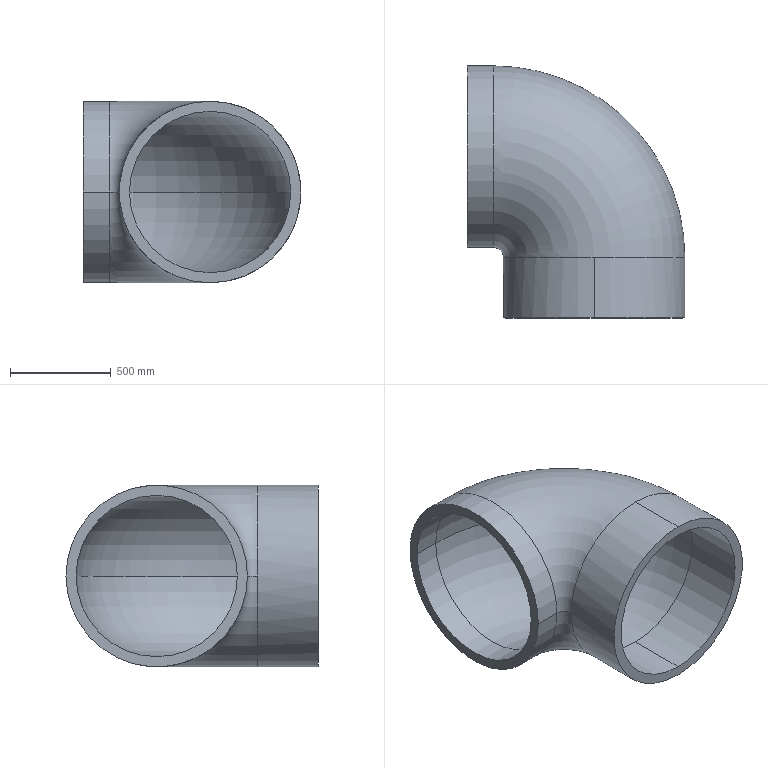Part | SolidWorks | features ICE 3, MoveFace 3, Extrusion 1, Sweep 1 | 1 solid | 14 faces | box 1080 x 1250 x 900 mm | volume 162277153 mm3 | cylinder 8 | torus 4 | plane 2 | commonest cylinder face diameters 800 x4 900 x4
STEP:
#1=CARTESIAN_POINT('',(0.,500.,-400.));
#2=VERTEX_POINT('',#1);
#3=CARTESIAN_POINT('',(400.,500.,0.));
#4=VERTEX_POINT('',#3);
#5=CARTESIAN_POINT('',(0.,500.,0.));
#6=DIRECTION('',(0.,-1.,0.));
#7=DIRECTION('',(0.,0.,1.));
#8=AXIS2_PLACEMENT_3D('',#5,#6,#7);
#9=CIRCLE('',#8,400.);
#10=EDGE_CURVE('',#2,#4,#9,.T.);
#11=ORIENTED_EDGE('',*,*,#10,.T.);
#12=CARTESIAN_POINT('',(-500.,1400.,0.));
#13=VERTEX_POINT('',#12);
#14=CARTESIAN_POINT('',(-500.,500.,0.));
#15=DIRECTION('',(0.,0.,1.));
#16=DIRECTION('',(1.,0.,0.));
#17=AXIS2_PLACEMENT_3D('',#14,#15,#16);
#18=CIRCLE('',#17,900.);
#19=EDGE_CURVE('',#4,#13,#18,.T.);
#20=ORIENTED_EDGE('',*,*,#19,.T.);
#21=CARTESIAN_POINT('',(-500.,600.,0.));
#22=VERTEX_POINT('',#21);
#23=CARTESIAN_POINT('',(-500.,1000.,0.));
#24=DIRECTION('',(1.,0.,0.));
#25=DIRECTION('',(0.,0.,1.));
#26=AXIS2_PLACEMENT_3D('',#23,#24,#25);
#27=CIRCLE('',#26,400.);
#28=EDGE_CURVE('',#22,#13,#27,.T.);
#29=ORIENTED_EDGE('',*,*,#28,.F.);
#30=CARTESIAN_POINT('',(-400.,500.,0.));
#31=VERTEX_POINT('',#30);
#32=CARTESIAN_POINT('',(-500.,500.,0.));
#33=DIRECTION('',(0.,0.,1.));
#34=DIRECTION('',(1.,0.,0.));
#35=AXIS2_PLACEMENT_3D('',#32,#33,#34);
#36=CIRCLE('',#35,100.);
#37=EDGE_CURVE('',#31,#22,#36,.T.);
#38=ORIENTED_EDGE('',*,*,#37,.F.);
#39=CARTESIAN_POINT('',(0.,500.,0.));
#40=DIRECTION('',(0.,-1.,0.));
#41=DIRECTION('',(0.,0.,1.));
#42=AXIS2_PLACEMENT_3D('',#39,#40,#41);
#43=CIRCLE('',#42,400.);
#44=EDGE_CURVE('',#31,#2,#43,.T.);
#45=ORIENTED_EDGE('',*,*,#44,.T.);
#46=EDGE_LOOP('',(#11,#20,#29,#38,#45));
#47=FACE_OUTER_BOUND('',#46,.T.);
#48=CARTESIAN_POINT('',(-500.,500.,0.));
#49=DIRECTION('',(0.,0.,1.));
#50=DIRECTION('',(1.,0.,0.));
#51=AXIS2_PLACEMENT_3D('',#48,#49,#50);
#52=TOROIDAL_SURFACE('',#51,500.,400.);
#53=ADVANCED_FACE('',(#47),#52,.F.);
#54=CARTESIAN_POINT('',(0.,500.,450.));
#55=VERTEX_POINT('',#54);
#56=CARTESIAN_POINT('',(450.,500.,0.));
#57=VERTEX_POINT('',#56);
#58=CARTESIAN_POINT('',(0.,500.,0.));
#59=DIRECTION('',(0.,1.,0.));
#60=DIRECTION('',(0.,0.,1.));
#61=AXIS2_PLACEMENT_3D('',#58,#59,#60);
#62=CIRCLE('',#61,450.);
#63=EDGE_CURVE('',#55,#57,#62,.T.);
#64=ORIENTED_EDGE('',*,*,#63,.T.);
#65=CARTESIAN_POINT('',(-500.,1450.,0.));
#66=VERTEX_POINT('',#65);
#67=CARTESIAN_POINT('',(-500.,500.,0.));
#68=DIRECTION('',(0.,0.,1.));
#69=DIRECTION('',(1.,0.,0.));
#70=AXIS2_PLACEMENT_3D('',#67,#68,#69);
#71=CIRCLE('',#70,950.);
#72=EDGE_CURVE('',#57,#66,#71,.T.);
#73=ORIENTED_EDGE('',*,*,#72,.T.);
#74=CARTESIAN_POINT('',(-500.,550.,0.));
#75=VERTEX_POINT('',#74);
#76=CARTESIAN_POINT('',(-500.,1000.,0.));
#77=DIRECTION('',(-1.,0.,0.));
#78=DIRECTION('',(0.,0.,1.));
#79=AXIS2_PLACEMENT_3D('',#76,#77,#78);
#80=CIRCLE('',#79,450.);
#81=EDGE_CURVE('',#75,#66,#80,.T.);
#82=ORIENTED_EDGE('',*,*,#81,.F.);
#83=CARTESIAN_POINT('',(-450.,500.,0.));
#84=VERTEX_POINT('',#83);
#85=CARTESIAN_POINT('',(-500.,500.,0.));
#86=DIRECTION('',(0.,0.,1.));
#87=DIRECTION('',(1.,0.,0.));
#88=AXIS2_PLACEMENT_3D('',#85,#86,#87);
#89=CIRCLE('',#88,50.);
#90=EDGE_CURVE('',#84,#75,#89,.T.);
#91=ORIENTED_EDGE('',*,*,#90,.F.);
#92=CARTESIAN_POINT('',(0.,500.,0.));
#93=DIRECTION('',(0.,1.,0.));
#94=DIRECTION('',(0.,0.,1.));
#95=AXIS2_PLACEMENT_3D('',#92,#93,#94);
#96=CIRCLE('',#95,450.);
#97=EDGE_CURVE('',#84,#55,#96,.T.);
#98=ORIENTED_EDGE('',*,*,#97,.T.);
#99=EDGE_LOOP('',(#64,#73,#82,#91,#98));
#100=FACE_OUTER_BOUND('',#99,.T.);
#101=CARTESIAN_POINT('',(-500.,500.,0.));
#102=DIRECTION('',(0.,0.,1.));
#103=DIRECTION('',(1.,0.,0.));
#104=AXIS2_PLACEMENT_3D('',#101,#102,#103);
#105=TOROIDAL_SURFACE('',#104,500.,450.);
#106=ADVANCED_FACE('',(#100),#105,.T.);
#107=CARTESIAN_POINT('',(0.,500.,400.));
#108=VERTEX_POINT('',#107);
#109=CARTESIAN_POINT('',(0.,500.,0.));
#110=DIRECTION('',(0.,-1.,0.));
#111=DIRECTION('',(0.,0.,1.));
#112=AXIS2_PLACEMENT_3D('',#109,#110,#111);
#113=CIRCLE('',#112,400.);
#114=EDGE_CURVE('',#108,#31,#113,.T.);
#115=ORIENTED_EDGE('',*,*,#114,.F.);
#116=CARTESIAN_POINT('',(0.,200.,400.));
#117=VERTEX_POINT('',#116);
#118=CARTESIAN_POINT('',(0.,750.,400.));
#119=DIRECTION('',(0.,-1.,0.));
#120=VECTOR('',#119,1000.);
#121=LINE('',#118,#120);
#122=EDGE_CURVE('',#108,#117,#121,.T.);
#123=ORIENTED_EDGE('',*,*,#122,.T.);
#124=CARTESIAN_POINT('',(0.,200.,-400.));
#125=VERTEX_POINT('',#124);
#126=CARTESIAN_POINT('',(0.,200.,0.));
#127=DIRECTION('',(0.,1.,0.));
#128=DIRECTION('',(0.,0.,1.));
#129=AXIS2_PLACEMENT_3D('',#126,#127,#128);
#130=CIRCLE('',#129,400.);
#131=EDGE_CURVE('',#125,#117,#130,.T.);
#132=ORIENTED_EDGE('',*,*,#131,.F.);
#133=CARTESIAN_POINT('',(0.,750.,-400.));
#134=DIRECTION('',(0.,-1.,0.));
#135=VECTOR('',#134,1000.);
#136=LINE('',#133,#135);
#137=EDGE_CURVE('',#2,#125,#136,.T.);
#138=ORIENTED_EDGE('',*,*,#137,.F.);
#139=ORIENTED_EDGE('',*,*,#44,.F.);
#140=EDGE_LOOP('',(#115,#123,#132,#138,#139));
#141=FACE_OUTER_BOUND('',#140,.T.);
#142=CARTESIAN_POINT('',(0.,750.,0.));
#143=DIRECTION('',(0.,-1.,0.));
#144=DIRECTION('',(0.,0.,-1.));
#145=AXIS2_PLACEMENT_3D('',#142,#143,#144);
#146=CYLINDRICAL_SURFACE('',#145,400.);
#147=ADVANCED_FACE('',(#141),#146,.F.);
#148=ORIENTED_EDGE('',*,*,#28,.T.);
#149=CARTESIAN_POINT('',(-630.,1400.,0.));
#150=VERTEX_POINT('',#149);
#151=CARTESIAN_POINT('',(-500.,1400.,0.));
#152=DIRECTION('',(-1.,0.,0.));
#153=VECTOR('',#152,1000.);
#154=LINE('',#151,#153);
#155=EDGE_CURVE('',#13,#150,#154,.T.);
#156=ORIENTED_EDGE('',*,*,#155,.T.);
#157=CARTESIAN_POINT('',(-630.,600.,0.));
#158=VERTEX_POINT('',#157);
#159=CARTESIAN_POINT('',(-630.,1000.,0.));
#160=DIRECTION('',(1.,0.,0.));
#161=DIRECTION('',(0.,0.,1.));
#162=AXIS2_PLACEMENT_3D('',#159,#160,#161);
#163=CIRCLE('',#162,400.);
#164=EDGE_CURVE('',#158,#150,#163,.T.);
#165=ORIENTED_EDGE('',*,*,#164,.F.);
#166=CARTESIAN_POINT('',(-500.,600.,0.));
#167=DIRECTION('',(-1.,0.,0.));
#168=VECTOR('',#167,1000.);
#169=LINE('',#166,#168);
#170=EDGE_CURVE('',#22,#158,#169,.T.);
#171=ORIENTED_EDGE('',*,*,#170,.F.);
#172=EDGE_LOOP('',(#148,#156,#165,#171));
#173=FACE_OUTER_BOUND('',#172,.T.);
#174=CARTESIAN_POINT('',(-500.,1000.,0.));
#175=DIRECTION('',(-1.,0.,0.));
#176=DIRECTION('',(0.,-1.,0.));
#177=AXIS2_PLACEMENT_3D('',#174,#175,#176);
#178=CYLINDRICAL_SURFACE('',#177,400.);
#179=ADVANCED_FACE('',(#173),#178,.F.);
#180=ORIENTED_EDGE('',*,*,#81,.T.);
#181=CARTESIAN_POINT('',(-630.,1450.,0.));
#182=VERTEX_POINT('',#181);
#183=CARTESIAN_POINT('',(-500.,1450.,0.));
#184=DIRECTION('',(-1.,0.,0.));
#185=VECTOR('',#184,1000.);
#186=LINE('',#183,#185);
#187=EDGE_CURVE('',#66,#182,#186,.T.);
#188=ORIENTED_EDGE('',*,*,#187,.T.);
#189=CARTESIAN_POINT('',(-630.,550.,0.));
#190=VERTEX_POINT('',#189);
#191=CARTESIAN_POINT('',(-630.,1000.,0.));
#192=DIRECTION('',(-1.,0.,0.));
#193=DIRECTION('',(0.,0.,1.));
#194=AXIS2_PLACEMENT_3D('',#191,#192,#193);
#195=CIRCLE('',#194,450.);
#196=EDGE_CURVE('',#190,#182,#195,.T.);
#197=ORIENTED_EDGE('',*,*,#196,.F.);
#198=CARTESIAN_POINT('',(-500.,550.,0.));
#199=DIRECTION('',(-1.,0.,0.));
#200=VECTOR('',#199,1000.);
#201=LINE('',#198,#200);
#202=EDGE_CURVE('',#75,#190,#201,.T.);
#203=ORIENTED_EDGE('',*,*,#202,.F.);
#204=EDGE_LOOP('',(#180,#188,#197,#203));
#205=FACE_OUTER_BOUND('',#204,.T.);
#206=CARTESIAN_POINT('',(-500.,1000.,0.));
#207=DIRECTION('',(-1.,0.,0.));
#208=DIRECTION('',(0.,-1.,0.));
#209=AXIS2_PLACEMENT_3D('',#206,#207,#208);
#210=CYLINDRICAL_SURFACE('',#209,450.);
#211=ADVANCED_FACE('',(#205),#210,.T.);
#212=ORIENTED_EDGE('',*,*,#63,.F.);
#213=CARTESIAN_POINT('',(0.,200.,450.));
#214=VERTEX_POINT('',#213);
#215=CARTESIAN_POINT('',(0.,750.,450.));
#216=DIRECTION('',(0.,-1.,0.));
#217=VECTOR('',#216,1000.);
#218=LINE('',#215,#217);
#219=EDGE_CURVE('',#55,#214,#218,.T.);
#220=ORIENTED_EDGE('',*,*,#219,.T.);
#221=CARTESIAN_POINT('',(0.,200.,-450.));
#222=VERTEX_POINT('',#221);
#223=CARTESIAN_POINT('',(0.,200.,0.));
#224=DIRECTION('',(0.,1.,0.));
#225=DIRECTION('',(0.,0.,1.));
#226=AXIS2_PLACEMENT_3D('',#223,#224,#225);
#227=CIRCLE('',#226,450.);
#228=EDGE_CURVE('',#214,#222,#227,.T.);
#229=ORIENTED_EDGE('',*,*,#228,.T.);
#230=CARTESIAN_POINT('',(0.,500.,-450.));
#231=VERTEX_POINT('',#230);
#232=CARTESIAN_POINT('',(0.,750.,-450.));
#233=DIRECTION('',(0.,-1.,0.));
#234=VECTOR('',#233,1000.);
#235=LINE('',#232,#234);
#236=EDGE_CURVE('',#231,#222,#235,.T.);
#237=ORIENTED_EDGE('',*,*,#236,.F.);
#238=CARTESIAN_POINT('',(0.,500.,0.));
#239=DIRECTION('',(0.,1.,0.));
#240=DIRECTION('',(0.,0.,1.));
#241=AXIS2_PLACEMENT_3D('',#238,#239,#240);
#242=CIRCLE('',#241,450.);
#243=EDGE_CURVE('',#57,#231,#242,.T.);
#244=ORIENTED_EDGE('',*,*,#243,.F.);
#245=EDGE_LOOP('',(#212,#220,#229,#237,#244));
#246=FACE_OUTER_BOUND('',#245,.T.);
#247=CARTESIAN_POINT('',(0.,750.,0.));
#248=DIRECTION('',(0.,-1.,0.));
#249=DIRECTION('',(0.,0.,-1.));
#250=AXIS2_PLACEMENT_3D('',#247,#248,#249);
#251=CYLINDRICAL_SURFACE('',#250,450.);
#252=ADVANCED_FACE('',(#246),#251,.T.);
#253=ORIENTED_EDGE('',*,*,#219,.F.);
#254=ORIENTED_EDGE('',*,*,#97,.F.);
#255=CARTESIAN_POINT('',(0.,500.,0.));
#256=DIRECTION('',(0.,1.,0.));
#257=DIRECTION('',(0.,0.,1.));
#258=AXIS2_PLACEMENT_3D('',#255,#256,#257);
#259=CIRCLE('',#258,450.);
#260=EDGE_CURVE('',#231,#84,#259,.T.);
#261=ORIENTED_EDGE('',*,*,#260,.F.);
#262=ORIENTED_EDGE('',*,*,#236,.T.);
#263=CARTESIAN_POINT('',(0.,200.,0.));
#264=DIRECTION('',(0.,1.,0.));
#265=DIRECTION('',(0.,0.,1.));
#266=AXIS2_PLACEMENT_3D('',#263,#264,#265);
#267=CIRCLE('',#266,450.);
#268=EDGE_CURVE('',#222,#214,#267,.T.);
#269=ORIENTED_EDGE('',*,*,#268,.T.);
#270=EDGE_LOOP('',(#253,#254,#261,#262,#269));
#271=FACE_OUTER_BOUND('',#270,.T.);
#272=CARTESIAN_POINT('',(0.,750.,0.));
#273=DIRECTION('',(0.,-1.,0.));
#274=DIRECTION('',(0.,0.,-1.));
#275=AXIS2_PLACEMENT_3D('',#272,#273,#274);
#276=CYLINDRICAL_SURFACE('',#275,450.);
#277=ADVANCED_FACE('',(#271),#276,.T.);
#278=ORIENTED_EDGE('',*,*,#155,.F.);
#279=CARTESIAN_POINT('',(-500.,1000.,0.));
#280=DIRECTION('',(1.,0.,0.));
#281=DIRECTION('',(0.,0.,1.));
#282=AXIS2_PLACEMENT_3D('',#279,#280,#281);
#283=CIRCLE('',#282,400.);
#284=EDGE_CURVE('',#13,#22,#283,.T.);
#285=ORIENTED_EDGE('',*,*,#284,.T.);
#286=ORIENTED_EDGE('',*,*,#170,.T.);
#287=CARTESIAN_POINT('',(-630.,1000.,0.));
#288=DIRECTION('',(1.,0.,0.));
#289=DIRECTION('',(0.,0.,1.));
#290=AXIS2_PLACEMENT_3D('',#287,#288,#289);
#291=CIRCLE('',#290,400.);
#292=EDGE_CURVE('',#150,#158,#291,.T.);
#293=ORIENTED_EDGE('',*,*,#292,.F.);
#294=EDGE_LOOP('',(#278,#285,#286,#293));
#295=FACE_OUTER_BOUND('',#294,.T.);
#296=CARTESIAN_POINT('',(-500.,1000.,0.));
#297=DIRECTION('',(-1.,0.,0.));
#298=DIRECTION('',(0.,-1.,0.));
#299=AXIS2_PLACEMENT_3D('',#296,#297,#298);
#300=CYLINDRICAL_SURFACE('',#299,400.);
#301=ADVANCED_FACE('',(#295),#300,.F.);
#302=ORIENTED_EDGE('',*,*,#19,.F.);
#303=CARTESIAN_POINT('',(0.,500.,0.));
#304=DIRECTION('',(0.,-1.,0.));
#305=DIRECTION('',(0.,0.,1.));
#306=AXIS2_PLACEMENT_3D('',#303,#304,#305);
#307=CIRCLE('',#306,400.);
#308=EDGE_CURVE('',#4,#108,#307,.T.);
#309=ORIENTED_EDGE('',*,*,#308,.T.);
#310=ORIENTED_EDGE('',*,*,#114,.T.);
#311=ORIENTED_EDGE('',*,*,#37,.T.);
#312=ORIENTED_EDGE('',*,*,#284,.F.);
#313=EDGE_LOOP('',(#302,#309,#310,#311,#312));
#314=FACE_OUTER_BOUND('',#313,.T.);
#315=CARTESIAN_POINT('',(-500.,500.,0.));
#316=DIRECTION('',(0.,0.,1.));
#317=DIRECTION('',(1.,0.,0.));
#318=AXIS2_PLACEMENT_3D('',#315,#316,#317);
#319=TOROIDAL_SURFACE('',#318,500.,400.);
#320=ADVANCED_FACE('',(#314),#319,.F.);
#321=ORIENTED_EDGE('',*,*,#164,.T.);
#322=ORIENTED_EDGE('',*,*,#292,.T.);
#323=EDGE_LOOP('',(#321,#322));
#324=FACE_BOUND('',#323,.T.);
#325=ORIENTED_EDGE('',*,*,#196,.T.);
#326=CARTESIAN_POINT('',(-630.,1000.,0.));
#327=DIRECTION('',(-1.,0.,0.));
#328=DIRECTION('',(0.,0.,1.));
#329=AXIS2_PLACEMENT_3D('',#326,#327,#328);
#330=CIRCLE('',#329,450.);
#331=EDGE_CURVE('',#182,#190,#330,.T.);
#332=ORIENTED_EDGE('',*,*,#331,.T.);
#333=EDGE_LOOP('',(#325,#332));
#334=FACE_OUTER_BOUND('',#333,.T.);
#335=CARTESIAN_POINT('',(-630.,1000.,0.));
#336=DIRECTION('',(-1.,0.,0.));
#337=DIRECTION('',(0.,0.,1.));
#338=AXIS2_PLACEMENT_3D('',#335,#336,#337);
#339=PLANE('',#338);
#340=ADVANCED_FACE('',(#324,#334),#339,.T.);
#341=ORIENTED_EDGE('',*,*,#187,.F.);
#342=CARTESIAN_POINT('',(-500.,1000.,0.));
#343=DIRECTION('',(-1.,0.,0.));
#344=DIRECTION('',(0.,0.,1.));
#345=AXIS2_PLACEMENT_3D('',#342,#343,#344);
#346=CIRCLE('',#345,450.);
#347=EDGE_CURVE('',#66,#75,#346,.T.);
#348=ORIENTED_EDGE('',*,*,#347,.T.);
#349=ORIENTED_EDGE('',*,*,#202,.T.);
#350=ORIENTED_EDGE('',*,*,#331,.F.);
#351=EDGE_LOOP('',(#341,#348,#349,#350));
#352=FACE_OUTER_BOUND('',#351,.T.);
#353=CARTESIAN_POINT('',(-500.,1000.,0.));
#354=DIRECTION('',(-1.,0.,0.));
#355=DIRECTION('',(0.,-1.,0.));
#356=AXIS2_PLACEMENT_3D('',#353,#354,#355);
#357=CYLINDRICAL_SURFACE('',#356,450.);
#358=ADVANCED_FACE('',(#352),#357,.T.);
#359=ORIENTED_EDGE('',*,*,#72,.F.);
#360=ORIENTED_EDGE('',*,*,#243,.T.);
#361=ORIENTED_EDGE('',*,*,#260,.T.);
#362=ORIENTED_EDGE('',*,*,#90,.T.);
#363=ORIENTED_EDGE('',*,*,#347,.F.);
#364=EDGE_LOOP('',(#359,#360,#361,#362,#363));
#365=FACE_OUTER_BOUND('',#364,.T.);
#366=CARTESIAN_POINT('',(-500.,500.,0.));
#367=DIRECTION('',(0.,0.,1.));
#368=DIRECTION('',(1.,0.,0.));
#369=AXIS2_PLACEMENT_3D('',#366,#367,#368);
#370=TOROIDAL_SURFACE('',#369,500.,450.);
#371=ADVANCED_FACE('',(#365),#370,.T.);
#372=ORIENTED_EDGE('',*,*,#122,.F.);
#373=ORIENTED_EDGE('',*,*,#308,.F.);
#374=ORIENTED_EDGE('',*,*,#10,.F.);
#375=ORIENTED_EDGE('',*,*,#137,.T.);
#376=CARTESIAN_POINT('',(0.,200.,0.));
#377=DIRECTION('',(0.,1.,0.));
#378=DIRECTION('',(0.,0.,1.));
#379=AXIS2_PLACEMENT_3D('',#376,#377,#378);
#380=CIRCLE('',#379,400.);
#381=EDGE_CURVE('',#117,#125,#380,.T.);
#382=ORIENTED_EDGE('',*,*,#381,.F.);
#383=EDGE_LOOP('',(#372,#373,#374,#375,#382));
#384=FACE_OUTER_BOUND('',#383,.T.);
#385=CARTESIAN_POINT('',(0.,750.,0.));
#386=DIRECTION('',(0.,-1.,0.));
#387=DIRECTION('',(0.,0.,-1.));
#388=AXIS2_PLACEMENT_3D('',#385,#386,#387);
#389=CYLINDRICAL_SURFACE('',#388,400.);
#390=ADVANCED_FACE('',(#384),#389,.F.);
#391=ORIENTED_EDGE('',*,*,#131,.T.);
#392=ORIENTED_EDGE('',*,*,#381,.T.);
#393=EDGE_LOOP('',(#391,#392));
#394=FACE_BOUND('',#393,.T.);
#395=ORIENTED_EDGE('',*,*,#268,.F.);
#396=ORIENTED_EDGE('',*,*,#228,.F.);
#397=EDGE_LOOP('',(#395,#396));
#398=FACE_OUTER_BOUND('',#397,.T.);
#399=CARTESIAN_POINT('',(-18.826,200.,0.));
#400=DIRECTION('',(0.,1.,0.));
#401=DIRECTION('',(0.,0.,1.));
#402=AXIS2_PLACEMENT_3D('',#399,#400,#401);
#403=PLANE('',#402);
#404=ADVANCED_FACE('',(#394,#398),#403,.F.);
#405=CLOSED_SHELL('',(#53,#106,#147,#179,#211,#252,#277,#301,#320,#340,#358,#371,#390,#404));
#406=MANIFOLD_SOLID_BREP('',#405);
#407=CARTESIAN_POINT('',(0.,0.,0.));
#408=DIRECTION('',(0.,0.,1.));
#409=DIRECTION('',(1.,0.,0.));
#410=AXIS2_PLACEMENT_3D('',#407,#408,#409);
#411=(LENGTH_UNIT()NAMED_UNIT(*)SI_UNIT(.MILLI.,.METRE.));
#412=UNCERTAINTY_MEASURE_WITH_UNIT(LENGTH_MEASURE(0.00001),#411,'','');
#413=(NAMED_UNIT(*)PLANE_ANGLE_UNIT()SI_UNIT($,.RADIAN.));
#414=(NAMED_UNIT(*)SI_UNIT($,.STERADIAN.)SOLID_ANGLE_UNIT());
#415=(GEOMETRIC_REPRESENTATION_CONTEXT(3)GLOBAL_UNCERTAINTY_ASSIGNED_CONTEXT((#412))GLOBAL_UNIT_ASSIGNED_CONTEXT((#411,#413,#414))REPRESENTATION_CONTEXT('',''));
#416=ADVANCED_BREP_SHAPE_REPRESENTATION('',(#406,#410),#415);